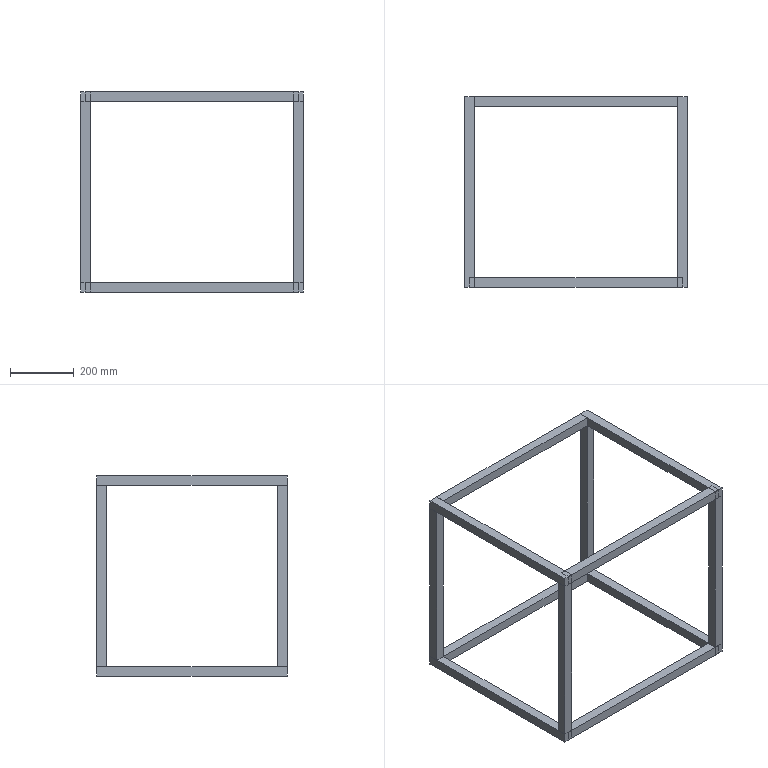Part | SolidWorks | features WeldMemberFeat 2, 3DProfileFeature 1, WeldCornerFeat 1, WeldmentFeature 1 | 12 solids | 72 faces | box 700 x 600 x 630 mm | volume 6570000 mm3 | plane 72